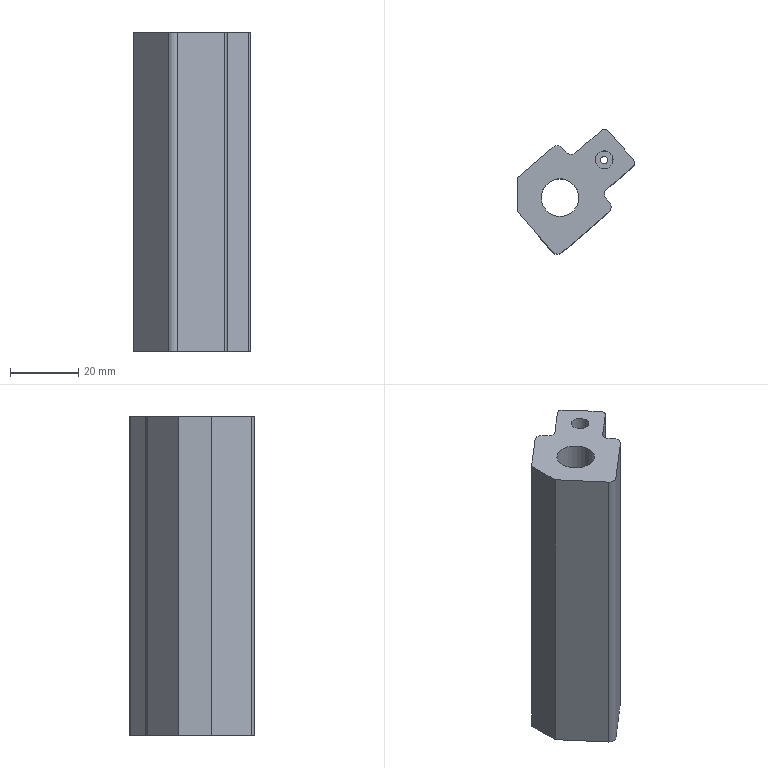Part | STEP file | gslz 2016.10.28-10_id2882_x_t | 1 solid | 24 faces | box 34.187 x 36.414 x 93 mm | volume 46333 mm3 | plane 12 | cylinder 11 | spline 1 | commonest cylinder face diameters 4 x5 3 x2 2.1 x1 5.2 x1 11 x1 17 x1